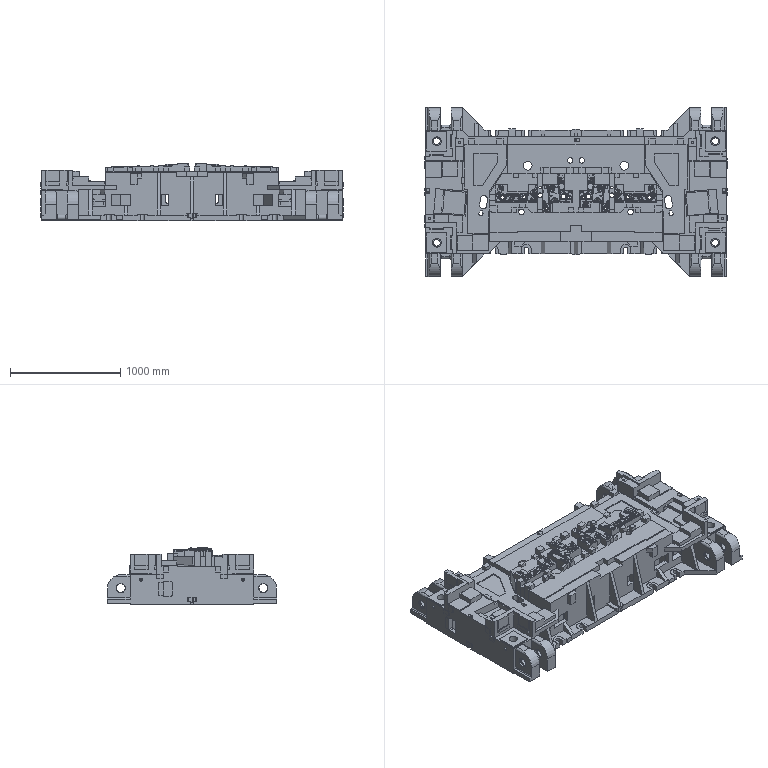Part | NX | features solid 2 | 1 solid | 2908 faces | box 2740 x 1530 x 517.599 mm | volume 502834432 mm3 | plane 1622 | spline 947 | cylinder 331 | torus 8 | commonest cylinder face diameters 60 x68 40 x50 83 x48 20 x25 4 x22 30 x18